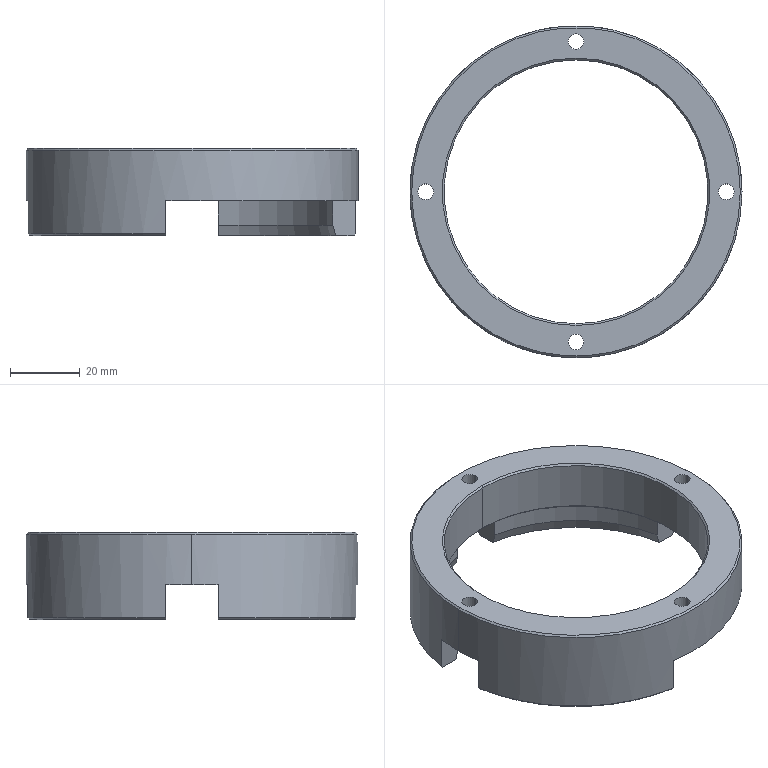Part | STEP file | PN_0005 JIG | 1 solid | 50 faces | box 95 x 95 x 25 mm | volume 47843 mm3 | cylinder 23 | plane 15 | cone 12 | commonest cylinder face diameters 4.5 x8 8 x8 82 x3 75.5 x2 95 x2